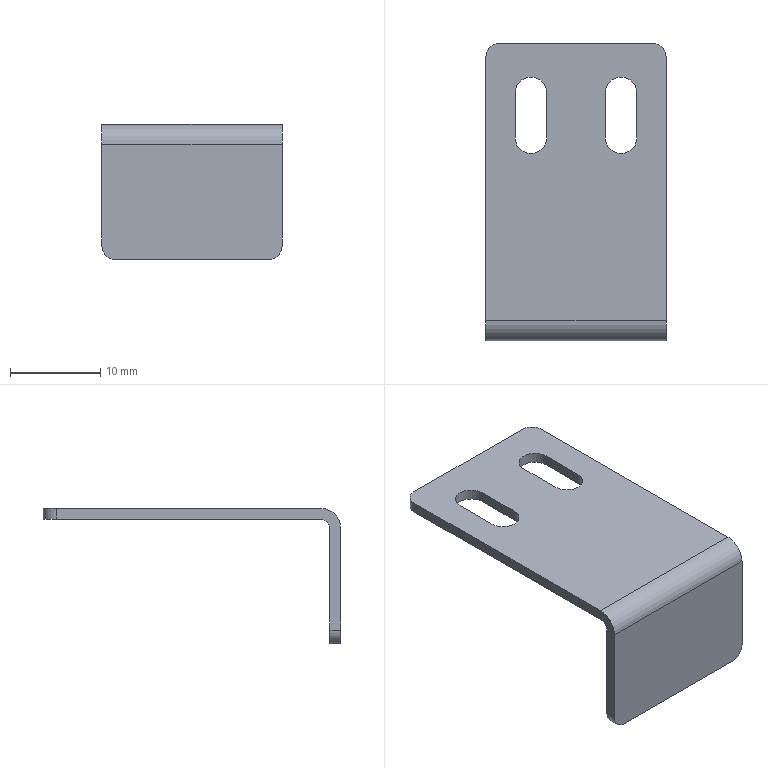Part | STEP file | Copy of K50-004 sensing plate^K50A-1H20-S(formula driven)-L300-motor left- | 1 solid | 22 faces | box 20 x 33 x 15 mm | volume 1039 mm3 | plane 12 | cylinder 10 | commonest cylinder face diameters 3 x4 3.5 x4 2 x1 4.4 x1